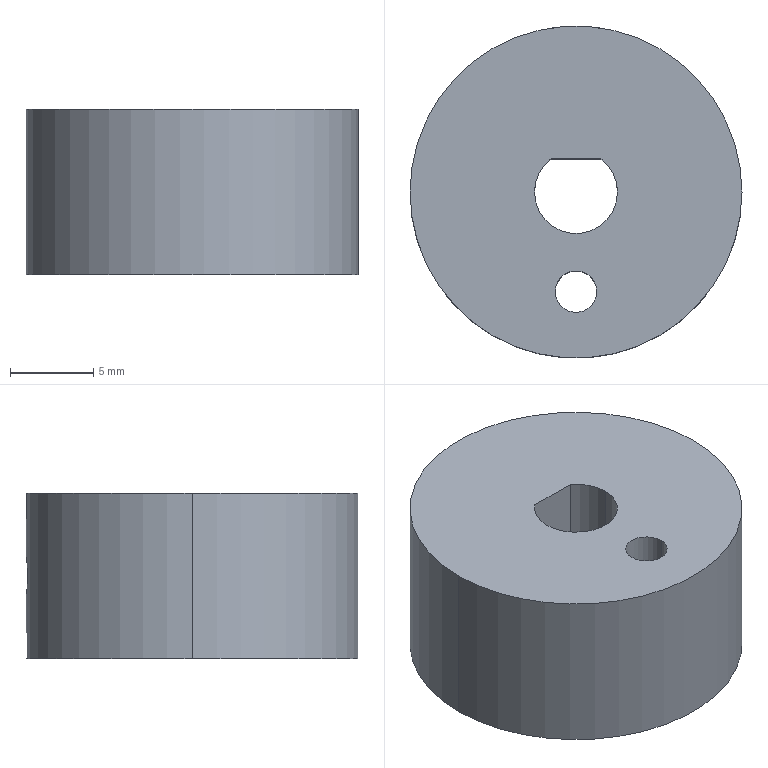Part | SolidWorks | features HoleWzd 2, Cut 1, Extrusion 1 | 1 solid | 12 faces | box 20 x 20 x 10 mm | volume 2867 mm3 | cylinder 9 | plane 3 | commonest cylinder face diameters 2.5 x4 5 x3 20 x2
STEP:
#1=CARTESIAN_POINT('',(1.25,-6.,10.));
#2=VERTEX_POINT('',#1);
#3=CARTESIAN_POINT('',(-1.25,-6.,10.));
#4=VERTEX_POINT('',#3);
#5=CARTESIAN_POINT('',(0.,-6.,10.));
#6=DIRECTION('',(0.,0.,-1.));
#7=DIRECTION('',(-1.,0.,0.));
#8=AXIS2_PLACEMENT_3D('',#5,#6,#7);
#9=CIRCLE('',#8,1.25);
#10=EDGE_CURVE('',#2,#4,#9,.T.);
#11=ORIENTED_EDGE('',*,*,#10,.F.);
#12=CARTESIAN_POINT('',(1.25,-6.,0.));
#13=VERTEX_POINT('',#12);
#14=CARTESIAN_POINT('',(1.25,-6.,0.));
#15=DIRECTION('',(0.,0.,-1.));
#16=VECTOR('',#15,1000.);
#17=LINE('',#14,#16);
#18=EDGE_CURVE('',#2,#13,#17,.T.);
#19=ORIENTED_EDGE('',*,*,#18,.T.);
#20=CARTESIAN_POINT('',(-1.25,-6.,0.));
#21=VERTEX_POINT('',#20);
#22=CARTESIAN_POINT('',(0.,-6.,0.));
#23=DIRECTION('',(0.,0.,-1.));
#24=DIRECTION('',(-1.,0.,0.));
#25=AXIS2_PLACEMENT_3D('',#22,#23,#24);
#26=CIRCLE('',#25,1.25);
#27=EDGE_CURVE('',#13,#21,#26,.T.);
#28=ORIENTED_EDGE('',*,*,#27,.T.);
#29=CARTESIAN_POINT('',(-1.25,-6.,0.));
#30=DIRECTION('',(0.,0.,-1.));
#31=VECTOR('',#30,1000.);
#32=LINE('',#29,#31);
#33=EDGE_CURVE('',#4,#21,#32,.T.);
#34=ORIENTED_EDGE('',*,*,#33,.F.);
#35=EDGE_LOOP('',(#11,#19,#28,#34));
#36=FACE_OUTER_BOUND('',#35,.T.);
#37=CARTESIAN_POINT('',(0.,-6.,0.));
#38=DIRECTION('',(0.,0.,-1.));
#39=DIRECTION('',(-1.,0.,0.));
#40=AXIS2_PLACEMENT_3D('',#37,#38,#39);
#41=CYLINDRICAL_SURFACE('',#40,1.25);
#42=ADVANCED_FACE('',(#36),#41,.F.);
#43=CARTESIAN_POINT('',(0.,2.,6.25));
#44=VERTEX_POINT('',#43);
#45=CARTESIAN_POINT('',(0.,2.,3.75));
#46=VERTEX_POINT('',#45);
#47=CARTESIAN_POINT('',(0.,2.,5.));
#48=DIRECTION('',(0.,-1.,0.));
#49=DIRECTION('',(0.,0.,-1.));
#50=AXIS2_PLACEMENT_3D('',#47,#48,#49);
#51=CIRCLE('',#50,1.25);
#52=EDGE_CURVE('',#44,#46,#51,.T.);
#53=ORIENTED_EDGE('',*,*,#52,.T.);
#54=CARTESIAN_POINT('',(0.,10.,3.75));
#55=VERTEX_POINT('',#54);
#56=CARTESIAN_POINT('',(0.,10.,3.75));
#57=DIRECTION('',(0.,1.,0.));
#58=VECTOR('',#57,1000.);
#59=LINE('',#56,#58);
#60=EDGE_CURVE('',#46,#55,#59,.T.);
#61=ORIENTED_EDGE('',*,*,#60,.T.);
#62=CARTESIAN_POINT('',(0.,10.,6.25));
#63=VERTEX_POINT('',#62);
#64=CARTESIAN_POINT('',(0.,10.,6.25));
#65=CARTESIAN_POINT('',(-0.1654,10.,6.25));
#66=CARTESIAN_POINT('',(-0.3276,9.996,6.217));
#67=CARTESIAN_POINT('',(-0.6303,9.981,6.092));
#68=CARTESIAN_POINT('',(-0.7689,9.971,5.999));
#69=CARTESIAN_POINT('',(-0.9992,9.951,5.768));
#70=CARTESIAN_POINT('',(-1.092,9.94,5.629));
#71=CARTESIAN_POINT('',(-1.217,9.926,5.328));
#72=CARTESIAN_POINT('',(-1.25,9.922,5.164));
#73=CARTESIAN_POINT('',(-1.25,9.922,4.919));
#74=CARTESIAN_POINT('',(-1.242,9.923,4.836));
#75=CARTESIAN_POINT('',(-1.21,9.927,4.676));
#76=CARTESIAN_POINT('',(-1.186,9.929,4.598));
#77=CARTESIAN_POINT('',(-1.092,9.94,4.37));
#78=CARTESIAN_POINT('',(-1.001,9.951,4.233));
#79=CARTESIAN_POINT('',(-0.7674,9.971,4.));
#80=CARTESIAN_POINT('',(-0.6298,9.981,3.908));
#81=CARTESIAN_POINT('',(-0.4028,9.992,3.814));
#82=CARTESIAN_POINT('',(-0.3249,9.995,3.79));
#83=CARTESIAN_POINT('',(-0.1645,9.999,3.758));
#84=CARTESIAN_POINT('',(-0.08162,10.,3.75));
#85=CARTESIAN_POINT('',(0.,10.,3.75));
#86=B_SPLINE_CURVE_WITH_KNOTS('',3,(#64,#65,#66,#67,#68,#69,#70,#71,#72,#73,#74,#75,#76,#77,#78,#79,#80,#81,#82,#83,#84,#85),.UNSPECIFIED.,.F.,.F.,(4,2,2,2,2,2,2,2,2,2,4),(0.,0.000489,0.000978,0.001467,0.001956,0.0022,0.002445,0.002934,0.003423,0.003667,0.003912),.UNSPECIFIED.);
#87=EDGE_CURVE('',#63,#55,#86,.T.);
#88=ORIENTED_EDGE('',*,*,#87,.F.);
#89=CARTESIAN_POINT('',(0.,10.,6.25));
#90=DIRECTION('',(0.,1.,0.));
#91=VECTOR('',#90,1000.);
#92=LINE('',#89,#91);
#93=EDGE_CURVE('',#44,#63,#92,.T.);
#94=ORIENTED_EDGE('',*,*,#93,.F.);
#95=EDGE_LOOP('',(#53,#61,#88,#94));
#96=FACE_OUTER_BOUND('',#95,.T.);
#97=CARTESIAN_POINT('',(0.,10.,5.));
#98=DIRECTION('',(0.,1.,0.));
#99=DIRECTION('',(0.,0.,1.));
#100=AXIS2_PLACEMENT_3D('',#97,#98,#99);
#101=CYLINDRICAL_SURFACE('',#100,1.25);
#102=ADVANCED_FACE('',(#96),#101,.F.);
#103=CARTESIAN_POINT('',(-2.5,0.,10.));
#104=VERTEX_POINT('',#103);
#105=CARTESIAN_POINT('',(2.5,0.,10.));
#106=VERTEX_POINT('',#105);
#107=CARTESIAN_POINT('',(0.,0.,10.));
#108=DIRECTION('',(0.,0.,1.));
#109=DIRECTION('',(0.,-1.,0.));
#110=AXIS2_PLACEMENT_3D('',#107,#108,#109);
#111=CIRCLE('',#110,2.5);
#112=EDGE_CURVE('',#104,#106,#111,.T.);
#113=ORIENTED_EDGE('',*,*,#112,.T.);
#114=CARTESIAN_POINT('',(2.5,0.,0.));
#115=VERTEX_POINT('',#114);
#116=CARTESIAN_POINT('',(2.5,0.,38.284));
#117=DIRECTION('',(0.,0.,-1.));
#118=VECTOR('',#117,1000.);
#119=LINE('',#116,#118);
#120=EDGE_CURVE('',#106,#115,#119,.T.);
#121=ORIENTED_EDGE('',*,*,#120,.T.);
#122=CARTESIAN_POINT('',(-2.5,0.,0.));
#123=VERTEX_POINT('',#122);
#124=CARTESIAN_POINT('',(0.,0.,0.));
#125=DIRECTION('',(0.,0.,1.));
#126=DIRECTION('',(1.,0.,0.));
#127=AXIS2_PLACEMENT_3D('',#124,#125,#126);
#128=CIRCLE('',#127,2.5);
#129=EDGE_CURVE('',#123,#115,#128,.T.);
#130=ORIENTED_EDGE('',*,*,#129,.F.);
#131=CARTESIAN_POINT('',(-2.5,0.,38.284));
#132=DIRECTION('',(0.,0.,-1.));
#133=VECTOR('',#132,1000.);
#134=LINE('',#131,#133);
#135=EDGE_CURVE('',#104,#123,#134,.T.);
#136=ORIENTED_EDGE('',*,*,#135,.F.);
#137=EDGE_LOOP('',(#113,#121,#130,#136));
#138=FACE_OUTER_BOUND('',#137,.T.);
#139=CARTESIAN_POINT('',(0.,0.,38.284));
#140=DIRECTION('',(0.,0.,-1.));
#141=DIRECTION('',(-1.,0.,0.));
#142=AXIS2_PLACEMENT_3D('',#139,#140,#141);
#143=CYLINDRICAL_SURFACE('',#142,2.5);
#144=ADVANCED_FACE('',(#138),#143,.F.);
#145=CARTESIAN_POINT('',(-1.5,2.,10.));
#146=VERTEX_POINT('',#145);
#147=CARTESIAN_POINT('',(0.,0.,10.));
#148=DIRECTION('',(0.,0.,1.));
#149=DIRECTION('',(0.,-1.,0.));
#150=AXIS2_PLACEMENT_3D('',#147,#148,#149);
#151=CIRCLE('',#150,2.5);
#152=EDGE_CURVE('',#146,#104,#151,.T.);
#153=ORIENTED_EDGE('',*,*,#152,.T.);
#154=ORIENTED_EDGE('',*,*,#135,.T.);
#155=CARTESIAN_POINT('',(-1.5,2.,0.));
#156=VERTEX_POINT('',#155);
#157=CARTESIAN_POINT('',(0.,0.,0.));
#158=DIRECTION('',(0.,0.,1.));
#159=DIRECTION('',(1.,0.,0.));
#160=AXIS2_PLACEMENT_3D('',#157,#158,#159);
#161=CIRCLE('',#160,2.5);
#162=EDGE_CURVE('',#156,#123,#161,.T.);
#163=ORIENTED_EDGE('',*,*,#162,.F.);
#164=CARTESIAN_POINT('',(-1.5,2.,38.284));
#165=DIRECTION('',(0.,0.,-1.));
#166=VECTOR('',#165,1000.);
#167=LINE('',#164,#166);
#168=EDGE_CURVE('',#146,#156,#167,.T.);
#169=ORIENTED_EDGE('',*,*,#168,.F.);
#170=EDGE_LOOP('',(#153,#154,#163,#169));
#171=FACE_OUTER_BOUND('',#170,.T.);
#172=CARTESIAN_POINT('',(0.,0.,38.284));
#173=DIRECTION('',(0.,0.,-1.));
#174=DIRECTION('',(-1.,0.,0.));
#175=AXIS2_PLACEMENT_3D('',#172,#173,#174);
#176=CYLINDRICAL_SURFACE('',#175,2.5);
#177=ADVANCED_FACE('',(#171),#176,.F.);
#178=ORIENTED_EDGE('',*,*,#87,.T.);
#179=CARTESIAN_POINT('',(0.,10.,3.75));
#180=CARTESIAN_POINT('',(0.1632,10.,3.75));
#181=CARTESIAN_POINT('',(0.3278,9.996,3.783));
#182=CARTESIAN_POINT('',(0.6287,9.981,3.907));
#183=CARTESIAN_POINT('',(0.768,9.971,4.));
#184=CARTESIAN_POINT('',(0.9986,9.951,4.231));
#185=CARTESIAN_POINT('',(1.091,9.94,4.369));
#186=CARTESIAN_POINT('',(1.217,9.926,4.672));
#187=CARTESIAN_POINT('',(1.25,9.922,4.834));
#188=CARTESIAN_POINT('',(1.25,9.922,5.164));
#189=CARTESIAN_POINT('',(1.218,9.926,5.327));
#190=CARTESIAN_POINT('',(1.092,9.94,5.629));
#191=CARTESIAN_POINT('',(0.9996,9.951,5.768));
#192=CARTESIAN_POINT('',(0.7694,9.971,5.999));
#193=CARTESIAN_POINT('',(0.6302,9.981,6.092));
#194=CARTESIAN_POINT('',(0.3296,9.996,6.217));
#195=CARTESIAN_POINT('',(0.1653,10.,6.25));
#196=CARTESIAN_POINT('',(0.,10.,6.25));
#197=B_SPLINE_CURVE_WITH_KNOTS('',3,(#179,#180,#181,#182,#183,#184,#185,#186,#187,#188,#189,#190,#191,#192,#193,#194,#195,#196),.UNSPECIFIED.,.F.,.F.,(4,2,2,2,2,2,2,2,4),(0.003912,0.004401,0.00489,0.005379,0.005867,0.006356,0.006845,0.007334,0.007823),.UNSPECIFIED.);
#198=EDGE_CURVE('',#55,#63,#197,.T.);
#199=ORIENTED_EDGE('',*,*,#198,.T.);
#200=EDGE_LOOP('',(#178,#199));
#201=FACE_BOUND('',#200,.T.);
#202=CARTESIAN_POINT('',(10.,0.,10.));
#203=VERTEX_POINT('',#202);
#204=CARTESIAN_POINT('',(-10.,0.,10.));
#205=VERTEX_POINT('',#204);
#206=CARTESIAN_POINT('',(0.,0.,10.));
#207=DIRECTION('',(0.,0.,1.));
#208=DIRECTION('',(0.,-1.,0.));
#209=AXIS2_PLACEMENT_3D('',#206,#207,#208);
#210=CIRCLE('',#209,10.);
#211=EDGE_CURVE('',#203,#205,#210,.T.);
#212=ORIENTED_EDGE('',*,*,#211,.F.);
#213=CARTESIAN_POINT('',(10.,0.,0.));
#214=VERTEX_POINT('',#213);
#215=CARTESIAN_POINT('',(10.,0.,38.284));
#216=DIRECTION('',(0.,0.,-1.));
#217=VECTOR('',#216,1000.);
#218=LINE('',#215,#217);
#219=EDGE_CURVE('',#203,#214,#218,.T.);
#220=ORIENTED_EDGE('',*,*,#219,.T.);
#221=CARTESIAN_POINT('',(-10.,0.,0.));
#222=VERTEX_POINT('',#221);
#223=CARTESIAN_POINT('',(0.,0.,0.));
#224=DIRECTION('',(0.,0.,1.));
#225=DIRECTION('',(1.,0.,0.));
#226=AXIS2_PLACEMENT_3D('',#223,#224,#225);
#227=CIRCLE('',#226,10.);
#228=EDGE_CURVE('',#214,#222,#227,.T.);
#229=ORIENTED_EDGE('',*,*,#228,.T.);
#230=CARTESIAN_POINT('',(-10.,0.,38.284));
#231=DIRECTION('',(0.,0.,-1.));
#232=VECTOR('',#231,1000.);
#233=LINE('',#230,#232);
#234=EDGE_CURVE('',#205,#222,#233,.T.);
#235=ORIENTED_EDGE('',*,*,#234,.F.);
#236=EDGE_LOOP('',(#212,#220,#229,#235));
#237=FACE_OUTER_BOUND('',#236,.T.);
#238=CARTESIAN_POINT('',(0.,0.,38.284));
#239=DIRECTION('',(0.,0.,-1.));
#240=DIRECTION('',(-1.,0.,0.));
#241=AXIS2_PLACEMENT_3D('',#238,#239,#240);
#242=CYLINDRICAL_SURFACE('',#241,10.);
#243=ADVANCED_FACE('',(#201,#237),#242,.T.);
#244=ORIENTED_EDGE('',*,*,#219,.F.);
#245=CARTESIAN_POINT('',(0.,0.,10.));
#246=DIRECTION('',(0.,0.,1.));
#247=DIRECTION('',(0.,-1.,0.));
#248=AXIS2_PLACEMENT_3D('',#245,#246,#247);
#249=CIRCLE('',#248,10.);
#250=EDGE_CURVE('',#205,#203,#249,.T.);
#251=ORIENTED_EDGE('',*,*,#250,.F.);
#252=ORIENTED_EDGE('',*,*,#234,.T.);
#253=CARTESIAN_POINT('',(0.,0.,0.));
#254=DIRECTION('',(0.,0.,1.));
#255=DIRECTION('',(1.,0.,0.));
#256=AXIS2_PLACEMENT_3D('',#253,#254,#255);
#257=CIRCLE('',#256,10.);
#258=EDGE_CURVE('',#222,#214,#257,.T.);
#259=ORIENTED_EDGE('',*,*,#258,.T.);
#260=EDGE_LOOP('',(#244,#251,#252,#259));
#261=FACE_OUTER_BOUND('',#260,.T.);
#262=CARTESIAN_POINT('',(0.,0.,38.284));
#263=DIRECTION('',(0.,0.,-1.));
#264=DIRECTION('',(-1.,0.,0.));
#265=AXIS2_PLACEMENT_3D('',#262,#263,#264);
#266=CYLINDRICAL_SURFACE('',#265,10.);
#267=ADVANCED_FACE('',(#261),#266,.T.);
#268=CARTESIAN_POINT('',(0.,-6.,0.));
#269=DIRECTION('',(0.,0.,-1.));
#270=DIRECTION('',(-1.,0.,0.));
#271=AXIS2_PLACEMENT_3D('',#268,#269,#270);
#272=CIRCLE('',#271,1.25);
#273=EDGE_CURVE('',#21,#13,#272,.T.);
#274=ORIENTED_EDGE('',*,*,#273,.F.);
#275=ORIENTED_EDGE('',*,*,#27,.F.);
#276=EDGE_LOOP('',(#274,#275));
#277=FACE_BOUND('',#276,.T.);
#278=ORIENTED_EDGE('',*,*,#258,.F.);
#279=ORIENTED_EDGE('',*,*,#228,.F.);
#280=EDGE_LOOP('',(#278,#279));
#281=FACE_OUTER_BOUND('',#280,.T.);
#282=ORIENTED_EDGE('',*,*,#162,.T.);
#283=ORIENTED_EDGE('',*,*,#129,.T.);
#284=CARTESIAN_POINT('',(1.5,2.,0.));
#285=VERTEX_POINT('',#284);
#286=CARTESIAN_POINT('',(0.,0.,0.));
#287=DIRECTION('',(0.,0.,1.));
#288=DIRECTION('',(1.,0.,0.));
#289=AXIS2_PLACEMENT_3D('',#286,#287,#288);
#290=CIRCLE('',#289,2.5);
#291=EDGE_CURVE('',#115,#285,#290,.T.);
#292=ORIENTED_EDGE('',*,*,#291,.T.);
#293=CARTESIAN_POINT('',(-1.5,2.,0.));
#294=DIRECTION('',(-1.,0.,0.));
#295=VECTOR('',#294,1000.);
#296=LINE('',#293,#295);
#297=EDGE_CURVE('',#285,#156,#296,.T.);
#298=ORIENTED_EDGE('',*,*,#297,.T.);
#299=EDGE_LOOP('',(#282,#283,#292,#298));
#300=FACE_BOUND('',#299,.T.);
#301=CARTESIAN_POINT('',(0.,0.,0.));
#302=DIRECTION('',(0.,0.,1.));
#303=DIRECTION('',(1.,0.,0.));
#304=AXIS2_PLACEMENT_3D('',#301,#302,#303);
#305=PLANE('',#304);
#306=ADVANCED_FACE('',(#277,#281,#300),#305,.F.);
#307=ORIENTED_EDGE('',*,*,#52,.F.);
#308=CARTESIAN_POINT('',(0.,2.,5.));
#309=DIRECTION('',(0.,-1.,0.));
#310=DIRECTION('',(0.,0.,-1.));
#311=AXIS2_PLACEMENT_3D('',#308,#309,#310);
#312=CIRCLE('',#311,1.25);
#313=EDGE_CURVE('',#46,#44,#312,.T.);
#314=ORIENTED_EDGE('',*,*,#313,.F.);
#315=EDGE_LOOP('',(#307,#314));
#316=FACE_BOUND('',#315,.T.);
#317=CARTESIAN_POINT('',(1.5,2.,10.));
#318=VERTEX_POINT('',#317);
#319=CARTESIAN_POINT('',(1.5,2.,38.284));
#320=DIRECTION('',(0.,0.,-1.));
#321=VECTOR('',#320,1000.);
#322=LINE('',#319,#321);
#323=EDGE_CURVE('',#318,#285,#322,.T.);
#324=ORIENTED_EDGE('',*,*,#323,.F.);
#325=CARTESIAN_POINT('',(-1.5,2.,10.));
#326=DIRECTION('',(-1.,0.,0.));
#327=VECTOR('',#326,1000.);
#328=LINE('',#325,#327);
#329=EDGE_CURVE('',#318,#146,#328,.T.);
#330=ORIENTED_EDGE('',*,*,#329,.T.);
#331=ORIENTED_EDGE('',*,*,#168,.T.);
#332=ORIENTED_EDGE('',*,*,#297,.F.);
#333=EDGE_LOOP('',(#324,#330,#331,#332));
#334=FACE_OUTER_BOUND('',#333,.T.);
#335=CARTESIAN_POINT('',(-1.5,2.,38.284));
#336=DIRECTION('',(0.,-1.,0.));
#337=DIRECTION('',(0.,0.,-1.));
#338=AXIS2_PLACEMENT_3D('',#335,#336,#337);
#339=PLANE('',#338);
#340=ADVANCED_FACE('',(#316,#334),#339,.T.);
#341=ORIENTED_EDGE('',*,*,#120,.F.);
#342=CARTESIAN_POINT('',(0.,0.,10.));
#343=DIRECTION('',(0.,0.,1.));
#344=DIRECTION('',(0.,-1.,0.));
#345=AXIS2_PLACEMENT_3D('',#342,#343,#344);
#346=CIRCLE('',#345,2.5);
#347=EDGE_CURVE('',#106,#318,#346,.T.);
#348=ORIENTED_EDGE('',*,*,#347,.T.);
#349=ORIENTED_EDGE('',*,*,#323,.T.);
#350=ORIENTED_EDGE('',*,*,#291,.F.);
#351=EDGE_LOOP('',(#341,#348,#349,#350));
#352=FACE_OUTER_BOUND('',#351,.T.);
#353=CARTESIAN_POINT('',(0.,0.,38.284));
#354=DIRECTION('',(0.,0.,-1.));
#355=DIRECTION('',(-1.,0.,0.));
#356=AXIS2_PLACEMENT_3D('',#353,#354,#355);
#357=CYLINDRICAL_SURFACE('',#356,2.5);
#358=ADVANCED_FACE('',(#352),#357,.F.);
#359=CARTESIAN_POINT('',(0.,-6.,10.));
#360=DIRECTION('',(0.,0.,-1.));
#361=DIRECTION('',(-1.,0.,0.));
#362=AXIS2_PLACEMENT_3D('',#359,#360,#361);
#363=CIRCLE('',#362,1.25);
#364=EDGE_CURVE('',#4,#2,#363,.T.);
#365=ORIENTED_EDGE('',*,*,#364,.T.);
#366=ORIENTED_EDGE('',*,*,#10,.T.);
#367=EDGE_LOOP('',(#365,#366));
#368=FACE_BOUND('',#367,.T.);
#369=ORIENTED_EDGE('',*,*,#152,.F.);
#370=ORIENTED_EDGE('',*,*,#329,.F.);
#371=ORIENTED_EDGE('',*,*,#347,.F.);
#372=ORIENTED_EDGE('',*,*,#112,.F.);
#373=EDGE_LOOP('',(#369,#370,#371,#372));
#374=FACE_BOUND('',#373,.T.);
#375=ORIENTED_EDGE('',*,*,#250,.T.);
#376=ORIENTED_EDGE('',*,*,#211,.T.);
#377=EDGE_LOOP('',(#375,#376));
#378=FACE_OUTER_BOUND('',#377,.T.);
#379=CARTESIAN_POINT('',(0.,2.5,10.));
#380=DIRECTION('',(0.,0.,1.));
#381=DIRECTION('',(0.,-1.,0.));
#382=AXIS2_PLACEMENT_3D('',#379,#380,#381);
#383=PLANE('',#382);
#384=ADVANCED_FACE('',(#368,#374,#378),#383,.T.);
#385=ORIENTED_EDGE('',*,*,#60,.F.);
#386=ORIENTED_EDGE('',*,*,#313,.T.);
#387=ORIENTED_EDGE('',*,*,#93,.T.);
#388=ORIENTED_EDGE('',*,*,#198,.F.);
#389=EDGE_LOOP('',(#385,#386,#387,#388));
#390=FACE_OUTER_BOUND('',#389,.T.);
#391=CARTESIAN_POINT('',(0.,10.,5.));
#392=DIRECTION('',(0.,1.,0.));
#393=DIRECTION('',(0.,0.,1.));
#394=AXIS2_PLACEMENT_3D('',#391,#392,#393);
#395=CYLINDRICAL_SURFACE('',#394,1.25);
#396=ADVANCED_FACE('',(#390),#395,.F.);
#397=ORIENTED_EDGE('',*,*,#18,.F.);
#398=ORIENTED_EDGE('',*,*,#364,.F.);
#399=ORIENTED_EDGE('',*,*,#33,.T.);
#400=ORIENTED_EDGE('',*,*,#273,.T.);
#401=EDGE_LOOP('',(#397,#398,#399,#400));
#402=FACE_OUTER_BOUND('',#401,.T.);
#403=CARTESIAN_POINT('',(0.,-6.,0.));
#404=DIRECTION('',(0.,0.,-1.));
#405=DIRECTION('',(-1.,0.,0.));
#406=AXIS2_PLACEMENT_3D('',#403,#404,#405);
#407=CYLINDRICAL_SURFACE('',#406,1.25);
#408=ADVANCED_FACE('',(#402),#407,.F.);
#409=CLOSED_SHELL('',(#42,#102,#144,#177,#243,#267,#306,#340,#358,#384,#396,#408));
#410=MANIFOLD_SOLID_BREP('',#409);
#411=CARTESIAN_POINT('',(0.,0.,0.));
#412=DIRECTION('',(0.,0.,1.));
#413=DIRECTION('',(1.,0.,0.));
#414=AXIS2_PLACEMENT_3D('',#411,#412,#413);
#415=(LENGTH_UNIT()NAMED_UNIT(*)SI_UNIT(.MILLI.,.METRE.));
#416=UNCERTAINTY_MEASURE_WITH_UNIT(LENGTH_MEASURE(0.00001),#415,'','');
#417=(NAMED_UNIT(*)PLANE_ANGLE_UNIT()SI_UNIT($,.RADIAN.));
#418=(NAMED_UNIT(*)SI_UNIT($,.STERADIAN.)SOLID_ANGLE_UNIT());
#419=(GEOMETRIC_REPRESENTATION_CONTEXT(3)GLOBAL_UNCERTAINTY_ASSIGNED_CONTEXT((#416))GLOBAL_UNIT_ASSIGNED_CONTEXT((#415,#417,#418))REPRESENTATION_CONTEXT('',''));
#420=ADVANCED_BREP_SHAPE_REPRESENTATION('',(#410,#414),#419);